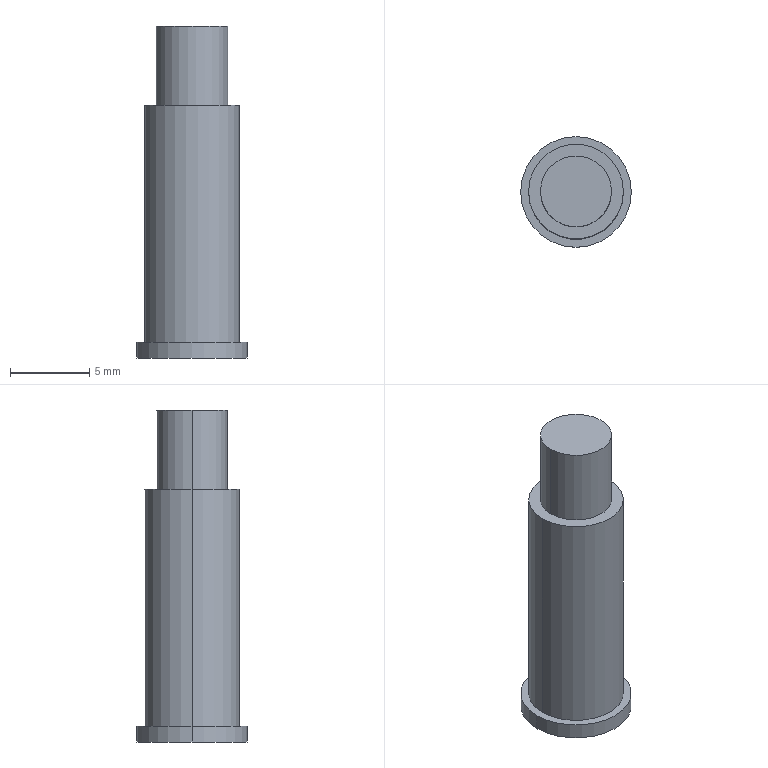Part | 1 solid | 10 faces | box 7 x 7 x 21 mm | volume 542.121 mm3 | cylinder 6 | plane 4 | commonest cylinder face diameters 4.5 x2 6 x2 7 x2
STEP:
#1=CARTESIAN_POINT('',(0.,0.,0.));
#2=DIRECTION('',(0.,0.,1.));
#3=DIRECTION('',(1.,0.,0.));
#4=AXIS2_PLACEMENT_3D('',#1,#2,#3);
#5=CARTESIAN_POINT('',(2.25,0.,16.));
#6=VERTEX_POINT('',#5);
#7=CARTESIAN_POINT('',(2.25,0.,21.));
#8=VERTEX_POINT('',#7);
#9=CARTESIAN_POINT('',(2.25,0.,18.5));
#10=DIRECTION('',(0.,0.,1.));
#11=VECTOR('',#10,1.);
#12=LINE('',#9,#11);
#13=CARTESIAN_POINT('',(0.,0.,18.5));
#14=DIRECTION('',(0.,0.,1.));
#15=DIRECTION('',(1.,0.,0.));
#16=AXIS2_PLACEMENT_3D('',#13,#14,#15);
#17=CYLINDRICAL_SURFACE('',#16,2.25);
#18=CARTESIAN_POINT('',(0.,0.));
#19=DIRECTION('',(0.,1.));
#20=VECTOR('',#19,1.);
#21=LINE('',#18,#20);
#22=(GEOMETRIC_REPRESENTATION_CONTEXT(2)PARAMETRIC_REPRESENTATION_CONTEXT()REPRESENTATION_CONTEXT('',''));
#23=DEFINITIONAL_REPRESENTATION('',(#21),#22);
#24=PCURVE('',#17,#23);
#25=CARTESIAN_POINT('',(0.,0.,18.5));
#26=DIRECTION('',(0.,0.,1.));
#27=DIRECTION('',(1.,0.,0.));
#28=AXIS2_PLACEMENT_3D('',#25,#26,#27);
#29=CYLINDRICAL_SURFACE('',#28,2.25);
#30=CARTESIAN_POINT('',(6.283,0.));
#31=DIRECTION('',(0.,1.));
#32=VECTOR('',#31,1.);
#33=LINE('',#30,#32);
#34=(GEOMETRIC_REPRESENTATION_CONTEXT(2)PARAMETRIC_REPRESENTATION_CONTEXT()REPRESENTATION_CONTEXT('',''));
#35=DEFINITIONAL_REPRESENTATION('',(#33),#34);
#36=PCURVE('',#29,#35);
#37=SURFACE_CURVE('',#12,(#24,#36),.PCURVE_S1.);
#38=EDGE_CURVE('',#6,#8,#37,.T.);
#39=ORIENTED_EDGE('',*,*,#38,.F.);
#40=CARTESIAN_POINT('',(-2.25,0.,16.));
#41=VERTEX_POINT('',#40);
#42=CARTESIAN_POINT('',(0.,0.,16.));
#43=DIRECTION('',(0.,0.,1.));
#44=DIRECTION('',(1.,0.,0.));
#45=AXIS2_PLACEMENT_3D('',#42,#43,#44);
#46=CIRCLE('',#45,2.25);
#47=CARTESIAN_POINT('',(0.,-2.5));
#48=DIRECTION('',(1.,0.));
#49=VECTOR('',#48,1.);
#50=LINE('',#47,#49);
#51=(GEOMETRIC_REPRESENTATION_CONTEXT(2)PARAMETRIC_REPRESENTATION_CONTEXT()REPRESENTATION_CONTEXT('',''));
#52=DEFINITIONAL_REPRESENTATION('',(#50),#51);
#53=PCURVE('',#17,#52);
#54=CARTESIAN_POINT('',(0.,0.,16.));
#55=DIRECTION('',(0.,0.,1.));
#56=DIRECTION('',(1.,0.,0.));
#57=AXIS2_PLACEMENT_3D('',#54,#55,#56);
#58=PLANE('',#57);
#59=CARTESIAN_POINT('',(0.,0.));
#60=DIRECTION('',(1.,0.));
#61=AXIS2_PLACEMENT_2D('',#59,#60);
#62=CIRCLE('',#61,2.25);
#63=(GEOMETRIC_REPRESENTATION_CONTEXT(2)PARAMETRIC_REPRESENTATION_CONTEXT()REPRESENTATION_CONTEXT('',''));
#64=DEFINITIONAL_REPRESENTATION('',(#62),#63);
#65=PCURVE('',#58,#64);
#66=SURFACE_CURVE('',#46,(#53,#65),.PCURVE_S1.);
#67=EDGE_CURVE('',#6,#41,#66,.T.);
#68=ORIENTED_EDGE('',*,*,#67,.T.);
#69=CARTESIAN_POINT('',(-2.25,0.,21.));
#70=VERTEX_POINT('',#69);
#71=CARTESIAN_POINT('',(-2.25,0.,18.5));
#72=DIRECTION('',(0.,0.,1.));
#73=VECTOR('',#72,1.);
#74=LINE('',#71,#73);
#75=CARTESIAN_POINT('',(3.142,0.));
#76=DIRECTION('',(0.,1.));
#77=VECTOR('',#76,1.);
#78=LINE('',#75,#77);
#79=(GEOMETRIC_REPRESENTATION_CONTEXT(2)PARAMETRIC_REPRESENTATION_CONTEXT()REPRESENTATION_CONTEXT('',''));
#80=DEFINITIONAL_REPRESENTATION('',(#78),#79);
#81=PCURVE('',#17,#80);
#82=CARTESIAN_POINT('',(3.142,0.));
#83=DIRECTION('',(0.,1.));
#84=VECTOR('',#83,1.);
#85=LINE('',#82,#84);
#86=(GEOMETRIC_REPRESENTATION_CONTEXT(2)PARAMETRIC_REPRESENTATION_CONTEXT()REPRESENTATION_CONTEXT('',''));
#87=DEFINITIONAL_REPRESENTATION('',(#85),#86);
#88=PCURVE('',#29,#87);
#89=SURFACE_CURVE('',#74,(#81,#88),.PCURVE_S1.);
#90=EDGE_CURVE('',#41,#70,#89,.T.);
#91=ORIENTED_EDGE('',*,*,#90,.T.);
#92=CARTESIAN_POINT('',(0.,0.,21.));
#93=DIRECTION('',(0.,0.,1.));
#94=DIRECTION('',(1.,0.,0.));
#95=AXIS2_PLACEMENT_3D('',#92,#93,#94);
#96=CIRCLE('',#95,2.25);
#97=CARTESIAN_POINT('',(0.,2.5));
#98=DIRECTION('',(1.,0.));
#99=VECTOR('',#98,1.);
#100=LINE('',#97,#99);
#101=(GEOMETRIC_REPRESENTATION_CONTEXT(2)PARAMETRIC_REPRESENTATION_CONTEXT()REPRESENTATION_CONTEXT('',''));
#102=DEFINITIONAL_REPRESENTATION('',(#100),#101);
#103=PCURVE('',#17,#102);
#104=CARTESIAN_POINT('',(0.,0.,21.));
#105=DIRECTION('',(0.,0.,1.));
#106=DIRECTION('',(1.,0.,0.));
#107=AXIS2_PLACEMENT_3D('',#104,#105,#106);
#108=PLANE('',#107);
#109=CARTESIAN_POINT('',(0.,0.));
#110=DIRECTION('',(1.,0.));
#111=AXIS2_PLACEMENT_2D('',#109,#110);
#112=CIRCLE('',#111,2.25);
#113=(GEOMETRIC_REPRESENTATION_CONTEXT(2)PARAMETRIC_REPRESENTATION_CONTEXT()REPRESENTATION_CONTEXT('',''));
#114=DEFINITIONAL_REPRESENTATION('',(#112),#113);
#115=PCURVE('',#108,#114);
#116=SURFACE_CURVE('',#96,(#103,#115),.PCURVE_S1.);
#117=EDGE_CURVE('',#8,#70,#116,.T.);
#118=ORIENTED_EDGE('',*,*,#117,.F.);
#119=EDGE_LOOP('',(#39,#68,#91,#118));
#120=FACE_BOUND('',#119,.T.);
#121=ADVANCED_FACE('',(#120),#17,.T.);
#122=ORIENTED_EDGE('',*,*,#90,.F.);
#123=CARTESIAN_POINT('',(0.,0.,16.));
#124=DIRECTION('',(0.,0.,1.));
#125=DIRECTION('',(1.,0.,0.));
#126=AXIS2_PLACEMENT_3D('',#123,#124,#125);
#127=CIRCLE('',#126,2.25);
#128=CARTESIAN_POINT('',(0.,-2.5));
#129=DIRECTION('',(1.,0.));
#130=VECTOR('',#129,1.);
#131=LINE('',#128,#130);
#132=(GEOMETRIC_REPRESENTATION_CONTEXT(2)PARAMETRIC_REPRESENTATION_CONTEXT()REPRESENTATION_CONTEXT('',''));
#133=DEFINITIONAL_REPRESENTATION('',(#131),#132);
#134=PCURVE('',#29,#133);
#135=CARTESIAN_POINT('',(0.,0.));
#136=DIRECTION('',(1.,0.));
#137=AXIS2_PLACEMENT_2D('',#135,#136);
#138=CIRCLE('',#137,2.25);
#139=(GEOMETRIC_REPRESENTATION_CONTEXT(2)PARAMETRIC_REPRESENTATION_CONTEXT()REPRESENTATION_CONTEXT('',''));
#140=DEFINITIONAL_REPRESENTATION('',(#138),#139);
#141=PCURVE('',#58,#140);
#142=SURFACE_CURVE('',#127,(#134,#141),.PCURVE_S1.);
#143=EDGE_CURVE('',#41,#6,#142,.T.);
#144=ORIENTED_EDGE('',*,*,#143,.T.);
#145=ORIENTED_EDGE('',*,*,#38,.T.);
#146=CARTESIAN_POINT('',(0.,0.,21.));
#147=DIRECTION('',(0.,0.,1.));
#148=DIRECTION('',(1.,0.,0.));
#149=AXIS2_PLACEMENT_3D('',#146,#147,#148);
#150=CIRCLE('',#149,2.25);
#151=CARTESIAN_POINT('',(0.,2.5));
#152=DIRECTION('',(1.,0.));
#153=VECTOR('',#152,1.);
#154=LINE('',#151,#153);
#155=(GEOMETRIC_REPRESENTATION_CONTEXT(2)PARAMETRIC_REPRESENTATION_CONTEXT()REPRESENTATION_CONTEXT('',''));
#156=DEFINITIONAL_REPRESENTATION('',(#154),#155);
#157=PCURVE('',#29,#156);
#158=CARTESIAN_POINT('',(0.,0.));
#159=DIRECTION('',(1.,0.));
#160=AXIS2_PLACEMENT_2D('',#158,#159);
#161=CIRCLE('',#160,2.25);
#162=(GEOMETRIC_REPRESENTATION_CONTEXT(2)PARAMETRIC_REPRESENTATION_CONTEXT()REPRESENTATION_CONTEXT('',''));
#163=DEFINITIONAL_REPRESENTATION('',(#161),#162);
#164=PCURVE('',#108,#163);
#165=SURFACE_CURVE('',#150,(#157,#164),.PCURVE_S1.);
#166=EDGE_CURVE('',#70,#8,#165,.T.);
#167=ORIENTED_EDGE('',*,*,#166,.F.);
#168=EDGE_LOOP('',(#122,#144,#145,#167));
#169=FACE_BOUND('',#168,.T.);
#170=ADVANCED_FACE('',(#169),#29,.T.);
#171=ORIENTED_EDGE('',*,*,#117,.T.);
#172=ORIENTED_EDGE('',*,*,#166,.T.);
#173=EDGE_LOOP('',(#171,#172));
#174=FACE_BOUND('',#173,.T.);
#175=ADVANCED_FACE('',(#174),#108,.T.);
#176=CARTESIAN_POINT('',(3.,0.,16.));
#177=VERTEX_POINT('',#176);
#178=CARTESIAN_POINT('',(-3.,0.,16.));
#179=VERTEX_POINT('',#178);
#180=CARTESIAN_POINT('',(0.,0.,16.));
#181=DIRECTION('',(0.,0.,1.));
#182=DIRECTION('',(1.,0.,0.));
#183=AXIS2_PLACEMENT_3D('',#180,#181,#182);
#184=CIRCLE('',#183,3.);
#185=CARTESIAN_POINT('',(0.,0.));
#186=DIRECTION('',(1.,0.));
#187=AXIS2_PLACEMENT_2D('',#185,#186);
#188=CIRCLE('',#187,3.);
#189=(GEOMETRIC_REPRESENTATION_CONTEXT(2)PARAMETRIC_REPRESENTATION_CONTEXT()REPRESENTATION_CONTEXT('',''));
#190=DEFINITIONAL_REPRESENTATION('',(#188),#189);
#191=PCURVE('',#58,#190);
#192=CARTESIAN_POINT('',(0.,0.,8.5));
#193=DIRECTION('',(0.,0.,1.));
#194=DIRECTION('',(1.,0.,0.));
#195=AXIS2_PLACEMENT_3D('',#192,#193,#194);
#196=CYLINDRICAL_SURFACE('',#195,3.);
#197=CARTESIAN_POINT('',(0.,7.5));
#198=DIRECTION('',(1.,0.));
#199=VECTOR('',#198,1.);
#200=LINE('',#197,#199);
#201=(GEOMETRIC_REPRESENTATION_CONTEXT(2)PARAMETRIC_REPRESENTATION_CONTEXT()REPRESENTATION_CONTEXT('',''));
#202=DEFINITIONAL_REPRESENTATION('',(#200),#201);
#203=PCURVE('',#196,#202);
#204=SURFACE_CURVE('',#184,(#191,#203),.PCURVE_S1.);
#205=EDGE_CURVE('',#177,#179,#204,.T.);
#206=ORIENTED_EDGE('',*,*,#205,.T.);
#207=CARTESIAN_POINT('',(0.,0.,16.));
#208=DIRECTION('',(0.,0.,1.));
#209=DIRECTION('',(1.,0.,0.));
#210=AXIS2_PLACEMENT_3D('',#207,#208,#209);
#211=CIRCLE('',#210,3.);
#212=CARTESIAN_POINT('',(0.,0.));
#213=DIRECTION('',(1.,0.));
#214=AXIS2_PLACEMENT_2D('',#212,#213);
#215=CIRCLE('',#214,3.);
#216=(GEOMETRIC_REPRESENTATION_CONTEXT(2)PARAMETRIC_REPRESENTATION_CONTEXT()REPRESENTATION_CONTEXT('',''));
#217=DEFINITIONAL_REPRESENTATION('',(#215),#216);
#218=PCURVE('',#58,#217);
#219=CARTESIAN_POINT('',(0.,0.,8.5));
#220=DIRECTION('',(0.,0.,1.));
#221=DIRECTION('',(1.,0.,0.));
#222=AXIS2_PLACEMENT_3D('',#219,#220,#221);
#223=CYLINDRICAL_SURFACE('',#222,3.);
#224=CARTESIAN_POINT('',(0.,7.5));
#225=DIRECTION('',(1.,0.));
#226=VECTOR('',#225,1.);
#227=LINE('',#224,#226);
#228=(GEOMETRIC_REPRESENTATION_CONTEXT(2)PARAMETRIC_REPRESENTATION_CONTEXT()REPRESENTATION_CONTEXT('',''));
#229=DEFINITIONAL_REPRESENTATION('',(#227),#228);
#230=PCURVE('',#223,#229);
#231=SURFACE_CURVE('',#211,(#218,#230),.PCURVE_S1.);
#232=EDGE_CURVE('',#179,#177,#231,.T.);
#233=ORIENTED_EDGE('',*,*,#232,.T.);
#234=EDGE_LOOP('',(#206,#233));
#235=FACE_BOUND('',#234,.T.);
#236=ORIENTED_EDGE('',*,*,#67,.F.);
#237=ORIENTED_EDGE('',*,*,#143,.F.);
#238=EDGE_LOOP('',(#236,#237));
#239=FACE_BOUND('',#238,.T.);
#240=ADVANCED_FACE('',(#235,#239),#58,.T.);
#241=CARTESIAN_POINT('',(3.5,0.,0.));
#242=VERTEX_POINT('',#241);
#243=CARTESIAN_POINT('',(3.5,0.,1.));
#244=VERTEX_POINT('',#243);
#245=CARTESIAN_POINT('',(3.5,0.,0.5));
#246=DIRECTION('',(0.,0.,1.));
#247=VECTOR('',#246,1.);
#248=LINE('',#245,#247);
#249=CARTESIAN_POINT('',(0.,0.,0.5));
#250=DIRECTION('',(0.,0.,1.));
#251=DIRECTION('',(1.,0.,0.));
#252=AXIS2_PLACEMENT_3D('',#249,#250,#251);
#253=CYLINDRICAL_SURFACE('',#252,3.5);
#254=CARTESIAN_POINT('',(0.,0.));
#255=DIRECTION('',(0.,1.));
#256=VECTOR('',#255,1.);
#257=LINE('',#254,#256);
#258=(GEOMETRIC_REPRESENTATION_CONTEXT(2)PARAMETRIC_REPRESENTATION_CONTEXT()REPRESENTATION_CONTEXT('',''));
#259=DEFINITIONAL_REPRESENTATION('',(#257),#258);
#260=PCURVE('',#253,#259);
#261=CARTESIAN_POINT('',(0.,0.,0.5));
#262=DIRECTION('',(0.,0.,1.));
#263=DIRECTION('',(1.,0.,0.));
#264=AXIS2_PLACEMENT_3D('',#261,#262,#263);
#265=CYLINDRICAL_SURFACE('',#264,3.5);
#266=CARTESIAN_POINT('',(6.283,0.));
#267=DIRECTION('',(0.,1.));
#268=VECTOR('',#267,1.);
#269=LINE('',#266,#268);
#270=(GEOMETRIC_REPRESENTATION_CONTEXT(2)PARAMETRIC_REPRESENTATION_CONTEXT()REPRESENTATION_CONTEXT('',''));
#271=DEFINITIONAL_REPRESENTATION('',(#269),#270);
#272=PCURVE('',#265,#271);
#273=SURFACE_CURVE('',#248,(#260,#272),.PCURVE_S1.);
#274=EDGE_CURVE('',#242,#244,#273,.T.);
#275=ORIENTED_EDGE('',*,*,#274,.F.);
#276=CARTESIAN_POINT('',(-3.5,0.,0.));
#277=VERTEX_POINT('',#276);
#278=CARTESIAN_POINT('',(0.,0.,0.));
#279=DIRECTION('',(0.,0.,1.));
#280=DIRECTION('',(1.,0.,0.));
#281=AXIS2_PLACEMENT_3D('',#278,#279,#280);
#282=CIRCLE('',#281,3.5);
#283=CARTESIAN_POINT('',(0.,-0.5));
#284=DIRECTION('',(1.,0.));
#285=VECTOR('',#284,1.);
#286=LINE('',#283,#285);
#287=(GEOMETRIC_REPRESENTATION_CONTEXT(2)PARAMETRIC_REPRESENTATION_CONTEXT()REPRESENTATION_CONTEXT('',''));
#288=DEFINITIONAL_REPRESENTATION('',(#286),#287);
#289=PCURVE('',#253,#288);
#290=CARTESIAN_POINT('',(0.,0.,0.));
#291=DIRECTION('',(0.,0.,1.));
#292=DIRECTION('',(1.,0.,0.));
#293=AXIS2_PLACEMENT_3D('',#290,#291,#292);
#294=PLANE('',#293);
#295=CARTESIAN_POINT('',(0.,0.));
#296=DIRECTION('',(1.,0.));
#297=AXIS2_PLACEMENT_2D('',#295,#296);
#298=CIRCLE('',#297,3.5);
#299=(GEOMETRIC_REPRESENTATION_CONTEXT(2)PARAMETRIC_REPRESENTATION_CONTEXT()REPRESENTATION_CONTEXT('',''));
#300=DEFINITIONAL_REPRESENTATION('',(#298),#299);
#301=PCURVE('',#294,#300);
#302=SURFACE_CURVE('',#282,(#289,#301),.PCURVE_S1.);
#303=EDGE_CURVE('',#242,#277,#302,.T.);
#304=ORIENTED_EDGE('',*,*,#303,.T.);
#305=CARTESIAN_POINT('',(-3.5,0.,1.));
#306=VERTEX_POINT('',#305);
#307=CARTESIAN_POINT('',(-3.5,0.,0.5));
#308=DIRECTION('',(0.,0.,1.));
#309=VECTOR('',#308,1.);
#310=LINE('',#307,#309);
#311=CARTESIAN_POINT('',(3.142,0.));
#312=DIRECTION('',(0.,1.));
#313=VECTOR('',#312,1.);
#314=LINE('',#311,#313);
#315=(GEOMETRIC_REPRESENTATION_CONTEXT(2)PARAMETRIC_REPRESENTATION_CONTEXT()REPRESENTATION_CONTEXT('',''));
#316=DEFINITIONAL_REPRESENTATION('',(#314),#315);
#317=PCURVE('',#253,#316);
#318=CARTESIAN_POINT('',(3.142,0.));
#319=DIRECTION('',(0.,1.));
#320=VECTOR('',#319,1.);
#321=LINE('',#318,#320);
#322=(GEOMETRIC_REPRESENTATION_CONTEXT(2)PARAMETRIC_REPRESENTATION_CONTEXT()REPRESENTATION_CONTEXT('',''));
#323=DEFINITIONAL_REPRESENTATION('',(#321),#322);
#324=PCURVE('',#265,#323);
#325=SURFACE_CURVE('',#310,(#317,#324),.PCURVE_S1.);
#326=EDGE_CURVE('',#277,#306,#325,.T.);
#327=ORIENTED_EDGE('',*,*,#326,.T.);
#328=CARTESIAN_POINT('',(0.,0.,1.));
#329=DIRECTION('',(0.,0.,1.));
#330=DIRECTION('',(1.,0.,0.));
#331=AXIS2_PLACEMENT_3D('',#328,#329,#330);
#332=CIRCLE('',#331,3.5);
#333=CARTESIAN_POINT('',(0.,0.5));
#334=DIRECTION('',(1.,0.));
#335=VECTOR('',#334,1.);
#336=LINE('',#333,#335);
#337=(GEOMETRIC_REPRESENTATION_CONTEXT(2)PARAMETRIC_REPRESENTATION_CONTEXT()REPRESENTATION_CONTEXT('',''));
#338=DEFINITIONAL_REPRESENTATION('',(#336),#337);
#339=PCURVE('',#253,#338);
#340=CARTESIAN_POINT('',(0.,0.,1.));
#341=DIRECTION('',(0.,0.,1.));
#342=DIRECTION('',(1.,0.,0.));
#343=AXIS2_PLACEMENT_3D('',#340,#341,#342);
#344=PLANE('',#343);
#345=CARTESIAN_POINT('',(0.,0.));
#346=DIRECTION('',(1.,0.));
#347=AXIS2_PLACEMENT_2D('',#345,#346);
#348=CIRCLE('',#347,3.5);
#349=(GEOMETRIC_REPRESENTATION_CONTEXT(2)PARAMETRIC_REPRESENTATION_CONTEXT()REPRESENTATION_CONTEXT('',''));
#350=DEFINITIONAL_REPRESENTATION('',(#348),#349);
#351=PCURVE('',#344,#350);
#352=SURFACE_CURVE('',#332,(#339,#351),.PCURVE_S1.);
#353=EDGE_CURVE('',#244,#306,#352,.T.);
#354=ORIENTED_EDGE('',*,*,#353,.F.);
#355=EDGE_LOOP('',(#275,#304,#327,#354));
#356=FACE_BOUND('',#355,.T.);
#357=ADVANCED_FACE('',(#356),#253,.T.);
#358=ORIENTED_EDGE('',*,*,#326,.F.);
#359=CARTESIAN_POINT('',(0.,0.,0.));
#360=DIRECTION('',(0.,0.,1.));
#361=DIRECTION('',(1.,0.,0.));
#362=AXIS2_PLACEMENT_3D('',#359,#360,#361);
#363=CIRCLE('',#362,3.5);
#364=CARTESIAN_POINT('',(0.,-0.5));
#365=DIRECTION('',(1.,0.));
#366=VECTOR('',#365,1.);
#367=LINE('',#364,#366);
#368=(GEOMETRIC_REPRESENTATION_CONTEXT(2)PARAMETRIC_REPRESENTATION_CONTEXT()REPRESENTATION_CONTEXT('',''));
#369=DEFINITIONAL_REPRESENTATION('',(#367),#368);
#370=PCURVE('',#265,#369);
#371=CARTESIAN_POINT('',(0.,0.));
#372=DIRECTION('',(1.,0.));
#373=AXIS2_PLACEMENT_2D('',#371,#372);
#374=CIRCLE('',#373,3.5);
#375=(GEOMETRIC_REPRESENTATION_CONTEXT(2)PARAMETRIC_REPRESENTATION_CONTEXT()REPRESENTATION_CONTEXT('',''));
#376=DEFINITIONAL_REPRESENTATION('',(#374),#375);
#377=PCURVE('',#294,#376);
#378=SURFACE_CURVE('',#363,(#370,#377),.PCURVE_S1.);
#379=EDGE_CURVE('',#277,#242,#378,.T.);
#380=ORIENTED_EDGE('',*,*,#379,.T.);
#381=ORIENTED_EDGE('',*,*,#274,.T.);
#382=CARTESIAN_POINT('',(0.,0.,1.));
#383=DIRECTION('',(0.,0.,1.));
#384=DIRECTION('',(1.,0.,0.));
#385=AXIS2_PLACEMENT_3D('',#382,#383,#384);
#386=CIRCLE('',#385,3.5);
#387=CARTESIAN_POINT('',(0.,0.5));
#388=DIRECTION('',(1.,0.));
#389=VECTOR('',#388,1.);
#390=LINE('',#387,#389);
#391=(GEOMETRIC_REPRESENTATION_CONTEXT(2)PARAMETRIC_REPRESENTATION_CONTEXT()REPRESENTATION_CONTEXT('',''));
#392=DEFINITIONAL_REPRESENTATION('',(#390),#391);
#393=PCURVE('',#265,#392);
#394=CARTESIAN_POINT('',(0.,0.));
#395=DIRECTION('',(1.,0.));
#396=AXIS2_PLACEMENT_2D('',#394,#395);
#397=CIRCLE('',#396,3.5);
#398=(GEOMETRIC_REPRESENTATION_CONTEXT(2)PARAMETRIC_REPRESENTATION_CONTEXT()REPRESENTATION_CONTEXT('',''));
#399=DEFINITIONAL_REPRESENTATION('',(#397),#398);
#400=PCURVE('',#344,#399);
#401=SURFACE_CURVE('',#386,(#393,#400),.PCURVE_S1.);
#402=EDGE_CURVE('',#306,#244,#401,.T.);
#403=ORIENTED_EDGE('',*,*,#402,.F.);
#404=EDGE_LOOP('',(#358,#380,#381,#403));
#405=FACE_BOUND('',#404,.T.);
#406=ADVANCED_FACE('',(#405),#265,.T.);
#407=ORIENTED_EDGE('',*,*,#379,.F.);
#408=ORIENTED_EDGE('',*,*,#303,.F.);
#409=EDGE_LOOP('',(#407,#408));
#410=FACE_BOUND('',#409,.T.);
#411=ADVANCED_FACE('',(#410),#294,.F.);
#412=ORIENTED_EDGE('',*,*,#353,.T.);
#413=ORIENTED_EDGE('',*,*,#402,.T.);
#414=EDGE_LOOP('',(#412,#413));
#415=FACE_BOUND('',#414,.T.);
#416=CARTESIAN_POINT('',(3.,0.,1.));
#417=VERTEX_POINT('',#416);
#418=CARTESIAN_POINT('',(-3.,0.,1.));
#419=VERTEX_POINT('',#418);
#420=CARTESIAN_POINT('',(0.,0.,1.));
#421=DIRECTION('',(0.,0.,1.));
#422=DIRECTION('',(1.,0.,0.));
#423=AXIS2_PLACEMENT_3D('',#420,#421,#422);
#424=CIRCLE('',#423,3.);
#425=CARTESIAN_POINT('',(0.,0.));
#426=DIRECTION('',(1.,0.));
#427=AXIS2_PLACEMENT_2D('',#425,#426);
#428=CIRCLE('',#427,3.);
#429=(GEOMETRIC_REPRESENTATION_CONTEXT(2)PARAMETRIC_REPRESENTATION_CONTEXT()REPRESENTATION_CONTEXT('',''));
#430=DEFINITIONAL_REPRESENTATION('',(#428),#429);
#431=PCURVE('',#344,#430);
#432=CARTESIAN_POINT('',(0.,-7.5));
#433=DIRECTION('',(1.,0.));
#434=VECTOR('',#433,1.);
#435=LINE('',#432,#434);
#436=(GEOMETRIC_REPRESENTATION_CONTEXT(2)PARAMETRIC_REPRESENTATION_CONTEXT()REPRESENTATION_CONTEXT('',''));
#437=DEFINITIONAL_REPRESENTATION('',(#435),#436);
#438=PCURVE('',#196,#437);
#439=SURFACE_CURVE('',#424,(#431,#438),.PCURVE_S1.);
#440=EDGE_CURVE('',#417,#419,#439,.T.);
#441=ORIENTED_EDGE('',*,*,#440,.F.);
#442=CARTESIAN_POINT('',(0.,0.,1.));
#443=DIRECTION('',(0.,0.,1.));
#444=DIRECTION('',(1.,0.,0.));
#445=AXIS2_PLACEMENT_3D('',#442,#443,#444);
#446=CIRCLE('',#445,3.);
#447=CARTESIAN_POINT('',(0.,0.));
#448=DIRECTION('',(1.,0.));
#449=AXIS2_PLACEMENT_2D('',#447,#448);
#450=CIRCLE('',#449,3.);
#451=(GEOMETRIC_REPRESENTATION_CONTEXT(2)PARAMETRIC_REPRESENTATION_CONTEXT()REPRESENTATION_CONTEXT('',''));
#452=DEFINITIONAL_REPRESENTATION('',(#450),#451);
#453=PCURVE('',#344,#452);
#454=CARTESIAN_POINT('',(0.,-7.5));
#455=DIRECTION('',(1.,0.));
#456=VECTOR('',#455,1.);
#457=LINE('',#454,#456);
#458=(GEOMETRIC_REPRESENTATION_CONTEXT(2)PARAMETRIC_REPRESENTATION_CONTEXT()REPRESENTATION_CONTEXT('',''));
#459=DEFINITIONAL_REPRESENTATION('',(#457),#458);
#460=PCURVE('',#223,#459);
#461=SURFACE_CURVE('',#446,(#453,#460),.PCURVE_S1.);
#462=EDGE_CURVE('',#419,#417,#461,.T.);
#463=ORIENTED_EDGE('',*,*,#462,.F.);
#464=EDGE_LOOP('',(#441,#463));
#465=FACE_BOUND('',#464,.T.);
#466=ADVANCED_FACE('',(#415,#465),#344,.T.);
#467=CARTESIAN_POINT('',(-3.,0.,8.5));
#468=DIRECTION('',(0.,0.,1.));
#469=VECTOR('',#468,1.);
#470=LINE('',#467,#469);
#471=CARTESIAN_POINT('',(3.142,0.));
#472=DIRECTION('',(0.,1.));
#473=VECTOR('',#472,1.);
#474=LINE('',#471,#473);
#475=(GEOMETRIC_REPRESENTATION_CONTEXT(2)PARAMETRIC_REPRESENTATION_CONTEXT()REPRESENTATION_CONTEXT('',''));
#476=DEFINITIONAL_REPRESENTATION('',(#474),#475);
#477=PCURVE('',#223,#476);
#478=CARTESIAN_POINT('',(3.142,0.));
#479=DIRECTION('',(0.,1.));
#480=VECTOR('',#479,1.);
#481=LINE('',#478,#480);
#482=(GEOMETRIC_REPRESENTATION_CONTEXT(2)PARAMETRIC_REPRESENTATION_CONTEXT()REPRESENTATION_CONTEXT('',''));
#483=DEFINITIONAL_REPRESENTATION('',(#481),#482);
#484=PCURVE('',#196,#483);
#485=SURFACE_CURVE('',#470,(#477,#484),.PCURVE_S1.);
#486=EDGE_CURVE('',#419,#179,#485,.T.);
#487=ORIENTED_EDGE('',*,*,#486,.F.);
#488=ORIENTED_EDGE('',*,*,#462,.T.);
#489=CARTESIAN_POINT('',(3.,0.,8.5));
#490=DIRECTION('',(0.,0.,1.));
#491=VECTOR('',#490,1.);
#492=LINE('',#489,#491);
#493=CARTESIAN_POINT('',(6.283,0.));
#494=DIRECTION('',(0.,1.));
#495=VECTOR('',#494,1.);
#496=LINE('',#493,#495);
#497=(GEOMETRIC_REPRESENTATION_CONTEXT(2)PARAMETRIC_REPRESENTATION_CONTEXT()REPRESENTATION_CONTEXT('',''));
#498=DEFINITIONAL_REPRESENTATION('',(#496),#497);
#499=PCURVE('',#223,#498);
#500=CARTESIAN_POINT('',(0.,0.));
#501=DIRECTION('',(0.,1.));
#502=VECTOR('',#501,1.);
#503=LINE('',#500,#502);
#504=(GEOMETRIC_REPRESENTATION_CONTEXT(2)PARAMETRIC_REPRESENTATION_CONTEXT()REPRESENTATION_CONTEXT('',''));
#505=DEFINITIONAL_REPRESENTATION('',(#503),#504);
#506=PCURVE('',#196,#505);
#507=SURFACE_CURVE('',#492,(#499,#506),.PCURVE_S1.);
#508=EDGE_CURVE('',#417,#177,#507,.T.);
#509=ORIENTED_EDGE('',*,*,#508,.T.);
#510=ORIENTED_EDGE('',*,*,#232,.F.);
#511=EDGE_LOOP('',(#487,#488,#509,#510));
#512=FACE_BOUND('',#511,.T.);
#513=ADVANCED_FACE('',(#512),#223,.T.);
#514=ORIENTED_EDGE('',*,*,#508,.F.);
#515=ORIENTED_EDGE('',*,*,#440,.T.);
#516=ORIENTED_EDGE('',*,*,#486,.T.);
#517=ORIENTED_EDGE('',*,*,#205,.F.);
#518=EDGE_LOOP('',(#514,#515,#516,#517));
#519=FACE_BOUND('',#518,.T.);
#520=ADVANCED_FACE('',(#519),#196,.T.);
#521=CLOSED_SHELL('',(#121,#170,#175,#240,#357,#406,#411,#466,#513,#520));
#522=MANIFOLD_SOLID_BREP('',#521);
#523=(LENGTH_UNIT()NAMED_UNIT(*)SI_UNIT(.MILLI.,.METRE.));
#524=UNCERTAINTY_MEASURE_WITH_UNIT(LENGTH_MEASURE(0.0000001),#523,'','');
#525=(NAMED_UNIT(*)PLANE_ANGLE_UNIT()SI_UNIT($,.RADIAN.));
#526=(NAMED_UNIT(*)SI_UNIT($,.STERADIAN.)SOLID_ANGLE_UNIT());
#527=(GEOMETRIC_REPRESENTATION_CONTEXT(3)GLOBAL_UNCERTAINTY_ASSIGNED_CONTEXT((#524))GLOBAL_UNIT_ASSIGNED_CONTEXT((#523,#525,#526))REPRESENTATION_CONTEXT('',''));
#528=ADVANCED_BREP_SHAPE_REPRESENTATION('',(#4,#522),#527);